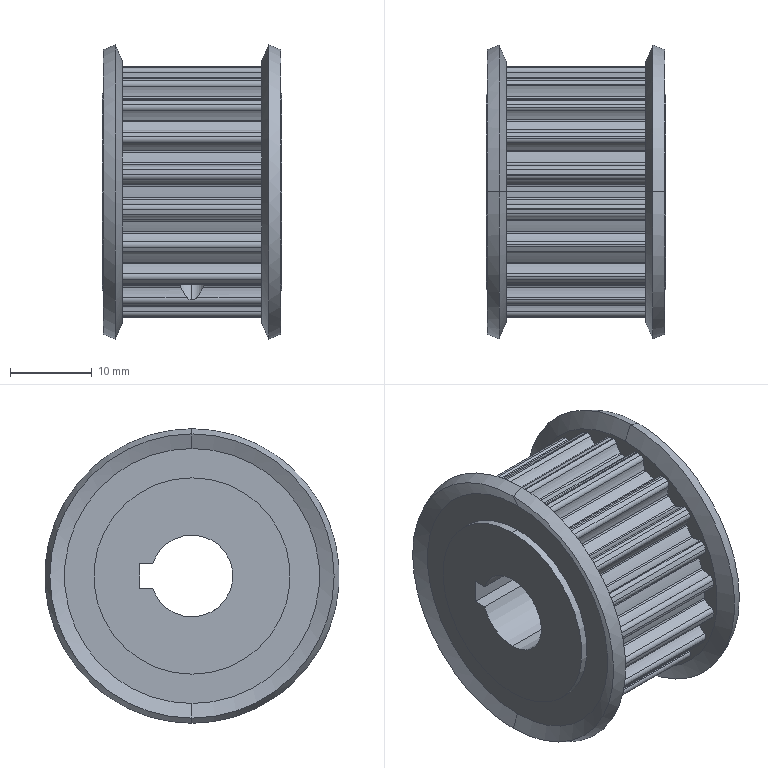Part | STEP file | 11-HTPA20S5M150_A_N10_a11 | 1 solid | 227 faces | box 22 x 36 x 36 mm | volume 13166 mm3 | cylinder 203 | cone 12 | plane 12 | commonest cylinder face diameters 0.5 x51 1.1 x50 6.55 x48 27.33 x23 30.87 x20 3.242 x4